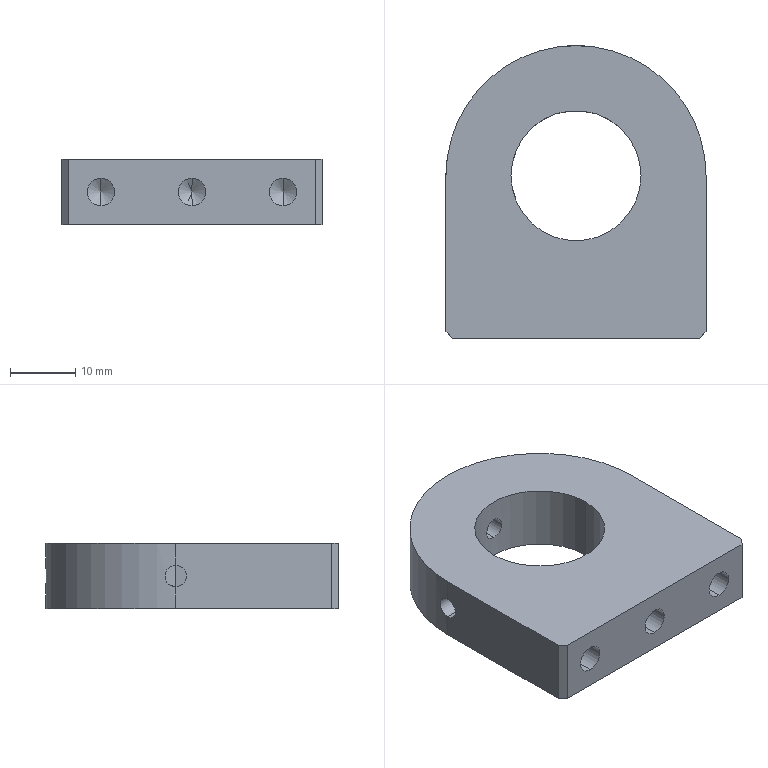Part | STEP file | MYT-A01-P11 | 1 solid | 27 faces | box 40 x 45 x 10 mm | volume 12427 mm3 | cylinder 14 | plane 7 | cone 6 | commonest cylinder face diameters 4.2 x6 3.3 x4 20 x2 40 x2
STEP:
#1=CARTESIAN_POINT('',(0.,35.,1.65));
#2=VERTEX_POINT('',#1);
#3=CARTESIAN_POINT('',(0.,35.,-1.65));
#4=VERTEX_POINT('',#3);
#5=CARTESIAN_POINT('',(0.,35.,1.65));
#6=CARTESIAN_POINT('',(-0.1092,35.,1.65));
#7=CARTESIAN_POINT('',(-0.2166,34.998,1.639));
#8=CARTESIAN_POINT('',(-0.4277,34.991,1.597));
#9=CARTESIAN_POINT('',(-0.5326,34.986,1.565));
#10=CARTESIAN_POINT('',(-0.7324,34.974,1.482));
#11=CARTESIAN_POINT('',(-0.8271,34.966,1.432));
#12=CARTESIAN_POINT('',(-1.006,34.95,1.312));
#13=CARTESIAN_POINT('',(-1.091,34.941,1.242));
#14=CARTESIAN_POINT('',(-1.319,34.914,1.014));
#15=CARTESIAN_POINT('',(-1.442,34.896,0.8307));
#16=CARTESIAN_POINT('',(-1.606,34.87,0.4337));
#17=CARTESIAN_POINT('',(-1.65,34.863,0.2163));
#18=CARTESIAN_POINT('',(-1.65,34.863,-0.1072));
#19=CARTESIAN_POINT('',(-1.639,34.865,-0.2167));
#20=CARTESIAN_POINT('',(-1.597,34.872,-0.4285));
#21=CARTESIAN_POINT('',(-1.566,34.877,-0.5315));
#22=CARTESIAN_POINT('',(-1.442,34.896,-0.8315));
#23=CARTESIAN_POINT('',(-1.32,34.914,-1.013));
#24=CARTESIAN_POINT('',(-1.09,34.941,-1.244));
#25=CARTESIAN_POINT('',(-1.007,34.95,-1.312));
#26=CARTESIAN_POINT('',(-0.8282,34.966,-1.431));
#27=CARTESIAN_POINT('',(-0.7316,34.974,-1.483));
#28=CARTESIAN_POINT('',(-0.532,34.986,-1.566));
#29=CARTESIAN_POINT('',(-0.4291,34.991,-1.597));
#30=CARTESIAN_POINT('',(-0.2173,34.998,-1.639));
#31=CARTESIAN_POINT('',(-0.1078,35.,-1.65));
#32=CARTESIAN_POINT('',(0.,35.,-1.65));
#33=B_SPLINE_CURVE_WITH_KNOTS('',3,(#5,#6,#7,#8,#9,#10,#11,#12,#13,#14,#15,#16,#17,#18,#19,#20,#21,#22,#23,#24,#25,#26,#27,#28,#29,#30,#31,#32),.UNSPECIFIED.,.F.,.F.,(4,2,2,2,2,2,2,2,2,2,2,2,2,4),(0.,0.000323,0.0006459,0.0009689,0.001292,0.001938,0.002584,0.002907,0.00323,0.003876,0.004199,0.004522,0.004845,0.005167),.UNSPECIFIED.);
#34=EDGE_CURVE('',#2,#4,#33,.T.);
#35=ORIENTED_EDGE('',*,*,#34,.T.);
#36=CARTESIAN_POINT('',(0.,45.,-1.65));
#37=VERTEX_POINT('',#36);
#38=CARTESIAN_POINT('',(0.,45.,-1.65));
#39=DIRECTION('',(0.,1.,0.));
#40=VECTOR('',#39,1000.);
#41=LINE('',#38,#40);
#42=EDGE_CURVE('',#4,#37,#41,.T.);
#43=ORIENTED_EDGE('',*,*,#42,.T.);
#44=CARTESIAN_POINT('',(0.,45.,1.65));
#45=VERTEX_POINT('',#44);
#46=CARTESIAN_POINT('',(0.,45.,-1.65));
#47=CARTESIAN_POINT('',(-0.109,45.,-1.65));
#48=CARTESIAN_POINT('',(-0.2163,44.999,-1.639));
#49=CARTESIAN_POINT('',(-0.4272,44.996,-1.597));
#50=CARTESIAN_POINT('',(-0.532,44.993,-1.566));
#51=CARTESIAN_POINT('',(-0.7318,44.987,-1.483));
#52=CARTESIAN_POINT('',(-0.8265,44.983,-1.432));
#53=CARTESIAN_POINT('',(-1.006,44.975,-1.312));
#54=CARTESIAN_POINT('',(-1.091,44.97,-1.243));
#55=CARTESIAN_POINT('',(-1.319,44.957,-1.015));
#56=CARTESIAN_POINT('',(-1.442,44.948,-0.8306));
#57=CARTESIAN_POINT('',(-1.606,44.936,-0.4336));
#58=CARTESIAN_POINT('',(-1.65,44.932,-0.2164));
#59=CARTESIAN_POINT('',(-1.65,44.932,0.1065));
#60=CARTESIAN_POINT('',(-1.639,44.933,0.2158));
#61=CARTESIAN_POINT('',(-1.597,44.936,0.4275));
#62=CARTESIAN_POINT('',(-1.566,44.939,0.5303));
#63=CARTESIAN_POINT('',(-1.484,44.945,0.7302));
#64=CARTESIAN_POINT('',(-1.432,44.949,0.8267));
#65=CARTESIAN_POINT('',(-1.313,44.957,1.006));
#66=CARTESIAN_POINT('',(-1.244,44.961,1.089));
#67=CARTESIAN_POINT('',(-1.091,44.97,1.243));
#68=CARTESIAN_POINT('',(-1.007,44.975,1.311));
#69=CARTESIAN_POINT('',(-0.8287,44.983,1.431));
#70=CARTESIAN_POINT('',(-0.7323,44.987,1.483));
#71=CARTESIAN_POINT('',(-0.4325,44.996,1.607));
#72=CARTESIAN_POINT('',(-0.2181,45.,1.65));
#73=CARTESIAN_POINT('',(0.,45.,1.65));
#74=B_SPLINE_CURVE_WITH_KNOTS('',3,(#46,#47,#48,#49,#50,#51,#52,#53,#54,#55,#56,#57,#58,#59,#60,#61,#62,#63,#64,#65,#66,#67,#68,#69,#70,#71,#72,#73),.UNSPECIFIED.,.F.,.F.,(4,2,2,2,2,2,2,2,2,2,2,2,2,4),(0.,0.0003225,0.000645,0.0009674,0.00129,0.001935,0.00258,0.002902,0.003225,0.003547,0.00387,0.004192,0.004515,0.00516),.UNSPECIFIED.);
#75=EDGE_CURVE('',#37,#45,#74,.T.);
#76=ORIENTED_EDGE('',*,*,#75,.T.);
#77=CARTESIAN_POINT('',(0.,45.,1.65));
#78=DIRECTION('',(0.,1.,0.));
#79=VECTOR('',#78,1000.);
#80=LINE('',#77,#79);
#81=EDGE_CURVE('',#2,#45,#80,.T.);
#82=ORIENTED_EDGE('',*,*,#81,.F.);
#83=EDGE_LOOP('',(#35,#43,#76,#82));
#84=FACE_OUTER_BOUND('',#83,.T.);
#85=CARTESIAN_POINT('',(0.,45.,0.));
#86=DIRECTION('',(0.,1.,0.));
#87=DIRECTION('',(0.,0.,1.));
#88=AXIS2_PLACEMENT_3D('',#85,#86,#87);
#89=CYLINDRICAL_SURFACE('',#88,1.65);
#90=ADVANCED_FACE('',(#84),#89,.F.);
#91=CARTESIAN_POINT('',(-10.,25.,1.65));
#92=VERTEX_POINT('',#91);
#93=CARTESIAN_POINT('',(-10.,25.,-1.65));
#94=VERTEX_POINT('',#93);
#95=CARTESIAN_POINT('',(-10.,25.,1.65));
#96=CARTESIAN_POINT('',(-10.,24.891,1.65));
#97=CARTESIAN_POINT('',(-9.998,24.783,1.639));
#98=CARTESIAN_POINT('',(-9.991,24.572,1.597));
#99=CARTESIAN_POINT('',(-9.986,24.467,1.565));
#100=CARTESIAN_POINT('',(-9.974,24.268,1.482));
#101=CARTESIAN_POINT('',(-9.966,24.173,1.432));
#102=CARTESIAN_POINT('',(-9.95,23.994,1.312));
#103=CARTESIAN_POINT('',(-9.941,23.909,1.242));
#104=CARTESIAN_POINT('',(-9.914,23.681,1.014));
#105=CARTESIAN_POINT('',(-9.896,23.558,0.8307));
#106=CARTESIAN_POINT('',(-9.87,23.394,0.4337));
#107=CARTESIAN_POINT('',(-9.863,23.35,0.2163));
#108=CARTESIAN_POINT('',(-9.863,23.35,-0.1072));
#109=CARTESIAN_POINT('',(-9.865,23.361,-0.2167));
#110=CARTESIAN_POINT('',(-9.872,23.403,-0.4285));
#111=CARTESIAN_POINT('',(-9.877,23.434,-0.5315));
#112=CARTESIAN_POINT('',(-9.896,23.558,-0.8315));
#113=CARTESIAN_POINT('',(-9.914,23.68,-1.013));
#114=CARTESIAN_POINT('',(-9.941,23.91,-1.244));
#115=CARTESIAN_POINT('',(-9.95,23.993,-1.312));
#116=CARTESIAN_POINT('',(-9.966,24.172,-1.431));
#117=CARTESIAN_POINT('',(-9.974,24.268,-1.483));
#118=CARTESIAN_POINT('',(-9.986,24.468,-1.566));
#119=CARTESIAN_POINT('',(-9.991,24.571,-1.597));
#120=CARTESIAN_POINT('',(-9.998,24.783,-1.639));
#121=CARTESIAN_POINT('',(-10.,24.892,-1.65));
#122=CARTESIAN_POINT('',(-10.,25.,-1.65));
#123=B_SPLINE_CURVE_WITH_KNOTS('',3,(#95,#96,#97,#98,#99,#100,#101,#102,#103,#104,#105,#106,#107,#108,#109,#110,#111,#112,#113,#114,#115,#116,#117,#118,#119,#120,#121,#122),.UNSPECIFIED.,.F.,.F.,(4,2,2,2,2,2,2,2,2,2,2,2,2,4),(0.,0.000323,0.0006459,0.0009689,0.001292,0.001938,0.002584,0.002907,0.00323,0.003876,0.004199,0.004522,0.004845,0.005167),.UNSPECIFIED.);
#124=EDGE_CURVE('',#92,#94,#123,.T.);
#125=ORIENTED_EDGE('',*,*,#124,.T.);
#126=CARTESIAN_POINT('',(-20.,25.,-1.65));
#127=VERTEX_POINT('',#126);
#128=CARTESIAN_POINT('',(-20.,25.,-1.65));
#129=DIRECTION('',(-1.,0.,0.));
#130=VECTOR('',#129,1000.);
#131=LINE('',#128,#130);
#132=EDGE_CURVE('',#94,#127,#131,.T.);
#133=ORIENTED_EDGE('',*,*,#132,.T.);
#134=CARTESIAN_POINT('',(-20.,25.,1.65));
#135=VERTEX_POINT('',#134);
#136=CARTESIAN_POINT('',(-20.,25.,0.));
#137=DIRECTION('',(-1.,0.,0.));
#138=DIRECTION('',(0.,0.,1.));
#139=AXIS2_PLACEMENT_3D('',#136,#137,#138);
#140=CIRCLE('',#139,1.65);
#141=EDGE_CURVE('',#127,#135,#140,.T.);
#142=ORIENTED_EDGE('',*,*,#141,.T.);
#143=CARTESIAN_POINT('',(-20.,25.,1.65));
#144=DIRECTION('',(-1.,0.,0.));
#145=VECTOR('',#144,1000.);
#146=LINE('',#143,#145);
#147=EDGE_CURVE('',#92,#135,#146,.T.);
#148=ORIENTED_EDGE('',*,*,#147,.F.);
#149=EDGE_LOOP('',(#125,#133,#142,#148));
#150=FACE_OUTER_BOUND('',#149,.T.);
#151=CARTESIAN_POINT('',(-20.,25.,0.));
#152=DIRECTION('',(-1.,0.,0.));
#153=DIRECTION('',(0.,0.,1.));
#154=AXIS2_PLACEMENT_3D('',#151,#152,#153);
#155=CYLINDRICAL_SURFACE('',#154,1.65);
#156=ADVANCED_FACE('',(#150),#155,.F.);
#157=CARTESIAN_POINT('',(-14.,12.4,2.1));
#158=VERTEX_POINT('',#157);
#159=CARTESIAN_POINT('',(-14.,12.4,-2.1));
#160=VERTEX_POINT('',#159);
#161=CARTESIAN_POINT('',(-14.,12.4,0.));
#162=DIRECTION('',(0.,-1.,0.));
#163=DIRECTION('',(0.,0.,-1.));
#164=AXIS2_PLACEMENT_3D('',#161,#162,#163);
#165=CIRCLE('',#164,2.1);
#166=EDGE_CURVE('',#158,#160,#165,.T.);
#167=ORIENTED_EDGE('',*,*,#166,.F.);
#168=CARTESIAN_POINT('',(-14.,0.,2.1));
#169=VERTEX_POINT('',#168);
#170=CARTESIAN_POINT('',(-14.,0.,2.1));
#171=DIRECTION('',(0.,-1.,0.));
#172=VECTOR('',#171,1000.);
#173=LINE('',#170,#172);
#174=EDGE_CURVE('',#158,#169,#173,.T.);
#175=ORIENTED_EDGE('',*,*,#174,.T.);
#176=CARTESIAN_POINT('',(-14.,0.,-2.1));
#177=VERTEX_POINT('',#176);
#178=CARTESIAN_POINT('',(-14.,0.,0.));
#179=DIRECTION('',(0.,-1.,0.));
#180=DIRECTION('',(0.,0.,-1.));
#181=AXIS2_PLACEMENT_3D('',#178,#179,#180);
#182=CIRCLE('',#181,2.1);
#183=EDGE_CURVE('',#169,#177,#182,.T.);
#184=ORIENTED_EDGE('',*,*,#183,.T.);
#185=CARTESIAN_POINT('',(-14.,0.,-2.1));
#186=DIRECTION('',(0.,-1.,0.));
#187=VECTOR('',#186,1000.);
#188=LINE('',#185,#187);
#189=EDGE_CURVE('',#160,#177,#188,.T.);
#190=ORIENTED_EDGE('',*,*,#189,.F.);
#191=EDGE_LOOP('',(#167,#175,#184,#190));
#192=FACE_OUTER_BOUND('',#191,.T.);
#193=CARTESIAN_POINT('',(-14.,0.,0.));
#194=DIRECTION('',(0.,-1.,0.));
#195=DIRECTION('',(0.,0.,-1.));
#196=AXIS2_PLACEMENT_3D('',#193,#194,#195);
#197=CYLINDRICAL_SURFACE('',#196,2.1);
#198=ADVANCED_FACE('',(#192),#197,.F.);
#199=CARTESIAN_POINT('',(-14.,13.662,0.));
#200=VERTEX_POINT('',#199);
#201=CARTESIAN_POINT('',(-14.,12.4,-2.1));
#202=DIRECTION('',(0.,-0.515,-0.8572));
#203=VECTOR('',#202,1000.);
#204=LINE('',#201,#203);
#205=EDGE_CURVE('',#200,#160,#204,.T.);
#206=ORIENTED_EDGE('',*,*,#205,.F.);
#207=CARTESIAN_POINT('',(-14.,12.4,2.1));
#208=DIRECTION('',(0.,-0.515,0.8572));
#209=VECTOR('',#208,1000.);
#210=LINE('',#207,#209);
#211=EDGE_CURVE('',#200,#158,#210,.T.);
#212=ORIENTED_EDGE('',*,*,#211,.T.);
#213=ORIENTED_EDGE('',*,*,#166,.T.);
#214=EDGE_LOOP('',(#206,#212,#213));
#215=FACE_OUTER_BOUND('',#214,.T.);
#216=CARTESIAN_POINT('',(-14.,12.4,0.));
#217=DIRECTION('',(0.,-1.,0.));
#218=DIRECTION('',(0.,0.,-1.));
#219=AXIS2_PLACEMENT_3D('',#216,#217,#218);
#220=CONICAL_SURFACE('',#219,2.1,1.03);
#221=ADVANCED_FACE('',(#215),#220,.F.);
#222=CARTESIAN_POINT('',(0.,12.4,2.1));
#223=VERTEX_POINT('',#222);
#224=CARTESIAN_POINT('',(0.,12.4,-2.1));
#225=VERTEX_POINT('',#224);
#226=CARTESIAN_POINT('',(0.,12.4,0.));
#227=DIRECTION('',(0.,-1.,0.));
#228=DIRECTION('',(0.,0.,-1.));
#229=AXIS2_PLACEMENT_3D('',#226,#227,#228);
#230=CIRCLE('',#229,2.1);
#231=EDGE_CURVE('',#223,#225,#230,.T.);
#232=ORIENTED_EDGE('',*,*,#231,.F.);
#233=CARTESIAN_POINT('',(0.,0.,2.1));
#234=VERTEX_POINT('',#233);
#235=CARTESIAN_POINT('',(0.,0.,2.1));
#236=DIRECTION('',(0.,-1.,0.));
#237=VECTOR('',#236,1000.);
#238=LINE('',#235,#237);
#239=EDGE_CURVE('',#223,#234,#238,.T.);
#240=ORIENTED_EDGE('',*,*,#239,.T.);
#241=CARTESIAN_POINT('',(0.,0.,-2.1));
#242=VERTEX_POINT('',#241);
#243=CARTESIAN_POINT('',(0.,0.,0.));
#244=DIRECTION('',(0.,-1.,0.));
#245=DIRECTION('',(0.,0.,-1.));
#246=AXIS2_PLACEMENT_3D('',#243,#244,#245);
#247=CIRCLE('',#246,2.1);
#248=EDGE_CURVE('',#234,#242,#247,.T.);
#249=ORIENTED_EDGE('',*,*,#248,.T.);
#250=CARTESIAN_POINT('',(0.,0.,-2.1));
#251=DIRECTION('',(0.,-1.,0.));
#252=VECTOR('',#251,1000.);
#253=LINE('',#250,#252);
#254=EDGE_CURVE('',#225,#242,#253,.T.);
#255=ORIENTED_EDGE('',*,*,#254,.F.);
#256=EDGE_LOOP('',(#232,#240,#249,#255));
#257=FACE_OUTER_BOUND('',#256,.T.);
#258=CARTESIAN_POINT('',(0.,0.,0.));
#259=DIRECTION('',(0.,-1.,0.));
#260=DIRECTION('',(0.,0.,-1.));
#261=AXIS2_PLACEMENT_3D('',#258,#259,#260);
#262=CYLINDRICAL_SURFACE('',#261,2.1);
#263=ADVANCED_FACE('',(#257),#262,.F.);
#264=CARTESIAN_POINT('',(0.,13.662,0.));
#265=VERTEX_POINT('',#264);
#266=CARTESIAN_POINT('',(0.,12.4,-2.1));
#267=DIRECTION('',(0.,-0.515,-0.8572));
#268=VECTOR('',#267,1000.);
#269=LINE('',#266,#268);
#270=EDGE_CURVE('',#265,#225,#269,.T.);
#271=ORIENTED_EDGE('',*,*,#270,.F.);
#272=CARTESIAN_POINT('',(0.,12.4,2.1));
#273=DIRECTION('',(0.,-0.515,0.8572));
#274=VECTOR('',#273,1000.);
#275=LINE('',#272,#274);
#276=EDGE_CURVE('',#265,#223,#275,.T.);
#277=ORIENTED_EDGE('',*,*,#276,.T.);
#278=ORIENTED_EDGE('',*,*,#231,.T.);
#279=EDGE_LOOP('',(#271,#277,#278));
#280=FACE_OUTER_BOUND('',#279,.T.);
#281=CARTESIAN_POINT('',(0.,12.4,0.));
#282=DIRECTION('',(0.,-1.,0.));
#283=DIRECTION('',(0.,0.,-1.));
#284=AXIS2_PLACEMENT_3D('',#281,#282,#283);
#285=CONICAL_SURFACE('',#284,2.1,1.03);
#286=ADVANCED_FACE('',(#280),#285,.F.);
#287=CARTESIAN_POINT('',(14.,12.4,2.1));
#288=VERTEX_POINT('',#287);
#289=CARTESIAN_POINT('',(14.,12.4,-2.1));
#290=VERTEX_POINT('',#289);
#291=CARTESIAN_POINT('',(14.,12.4,0.));
#292=DIRECTION('',(0.,-1.,0.));
#293=DIRECTION('',(0.,0.,-1.));
#294=AXIS2_PLACEMENT_3D('',#291,#292,#293);
#295=CIRCLE('',#294,2.1);
#296=EDGE_CURVE('',#288,#290,#295,.T.);
#297=ORIENTED_EDGE('',*,*,#296,.F.);
#298=CARTESIAN_POINT('',(14.,0.,2.1));
#299=VERTEX_POINT('',#298);
#300=CARTESIAN_POINT('',(14.,0.,2.1));
#301=DIRECTION('',(0.,-1.,0.));
#302=VECTOR('',#301,1000.);
#303=LINE('',#300,#302);
#304=EDGE_CURVE('',#288,#299,#303,.T.);
#305=ORIENTED_EDGE('',*,*,#304,.T.);
#306=CARTESIAN_POINT('',(14.,0.,-2.1));
#307=VERTEX_POINT('',#306);
#308=CARTESIAN_POINT('',(14.,0.,0.));
#309=DIRECTION('',(0.,-1.,0.));
#310=DIRECTION('',(0.,0.,-1.));
#311=AXIS2_PLACEMENT_3D('',#308,#309,#310);
#312=CIRCLE('',#311,2.1);
#313=EDGE_CURVE('',#299,#307,#312,.T.);
#314=ORIENTED_EDGE('',*,*,#313,.T.);
#315=CARTESIAN_POINT('',(14.,0.,-2.1));
#316=DIRECTION('',(0.,-1.,0.));
#317=VECTOR('',#316,1000.);
#318=LINE('',#315,#317);
#319=EDGE_CURVE('',#290,#307,#318,.T.);
#320=ORIENTED_EDGE('',*,*,#319,.F.);
#321=EDGE_LOOP('',(#297,#305,#314,#320));
#322=FACE_OUTER_BOUND('',#321,.T.);
#323=CARTESIAN_POINT('',(14.,0.,0.));
#324=DIRECTION('',(0.,-1.,0.));
#325=DIRECTION('',(0.,0.,-1.));
#326=AXIS2_PLACEMENT_3D('',#323,#324,#325);
#327=CYLINDRICAL_SURFACE('',#326,2.1);
#328=ADVANCED_FACE('',(#322),#327,.F.);
#329=CARTESIAN_POINT('',(14.,13.662,0.));
#330=VERTEX_POINT('',#329);
#331=CARTESIAN_POINT('',(14.,12.4,-2.1));
#332=DIRECTION('',(0.,-0.515,-0.8572));
#333=VECTOR('',#332,1000.);
#334=LINE('',#331,#333);
#335=EDGE_CURVE('',#330,#290,#334,.T.);
#336=ORIENTED_EDGE('',*,*,#335,.F.);
#337=CARTESIAN_POINT('',(14.,12.4,2.1));
#338=DIRECTION('',(0.,-0.515,0.8572));
#339=VECTOR('',#338,1000.);
#340=LINE('',#337,#339);
#341=EDGE_CURVE('',#330,#288,#340,.T.);
#342=ORIENTED_EDGE('',*,*,#341,.T.);
#343=ORIENTED_EDGE('',*,*,#296,.T.);
#344=EDGE_LOOP('',(#336,#342,#343));
#345=FACE_OUTER_BOUND('',#344,.T.);
#346=CARTESIAN_POINT('',(14.,12.4,0.));
#347=DIRECTION('',(0.,-1.,0.));
#348=DIRECTION('',(0.,0.,-1.));
#349=AXIS2_PLACEMENT_3D('',#346,#347,#348);
#350=CONICAL_SURFACE('',#349,2.1,1.03);
#351=ADVANCED_FACE('',(#345),#350,.F.);
#352=CARTESIAN_POINT('',(-10.,25.,5.));
#353=VERTEX_POINT('',#352);
#354=CARTESIAN_POINT('',(10.,25.,5.));
#355=VERTEX_POINT('',#354);
#356=CARTESIAN_POINT('',(0.,25.,5.));
#357=DIRECTION('',(0.,0.,1.));
#358=DIRECTION('',(1.,0.,0.));
#359=AXIS2_PLACEMENT_3D('',#356,#357,#358);
#360=CIRCLE('',#359,10.);
#361=EDGE_CURVE('',#353,#355,#360,.T.);
#362=ORIENTED_EDGE('',*,*,#361,.T.);
#363=CARTESIAN_POINT('',(10.,25.,-5.));
#364=VERTEX_POINT('',#363);
#365=CARTESIAN_POINT('',(10.,25.,5.));
#366=DIRECTION('',(0.,0.,-1.));
#367=VECTOR('',#366,1000.);
#368=LINE('',#365,#367);
#369=EDGE_CURVE('',#355,#364,#368,.T.);
#370=ORIENTED_EDGE('',*,*,#369,.T.);
#371=CARTESIAN_POINT('',(-10.,25.,-5.));
#372=VERTEX_POINT('',#371);
#373=CARTESIAN_POINT('',(0.,25.,-5.));
#374=DIRECTION('',(0.,0.,1.));
#375=DIRECTION('',(1.,0.,0.));
#376=AXIS2_PLACEMENT_3D('',#373,#374,#375);
#377=CIRCLE('',#376,10.);
#378=EDGE_CURVE('',#372,#364,#377,.T.);
#379=ORIENTED_EDGE('',*,*,#378,.F.);
#380=CARTESIAN_POINT('',(-10.,25.,5.));
#381=DIRECTION('',(0.,0.,-1.));
#382=VECTOR('',#381,1000.);
#383=LINE('',#380,#382);
#384=EDGE_CURVE('',#94,#372,#383,.T.);
#385=ORIENTED_EDGE('',*,*,#384,.F.);
#386=ORIENTED_EDGE('',*,*,#124,.F.);
#387=CARTESIAN_POINT('',(-10.,25.,5.));
#388=DIRECTION('',(0.,0.,-1.));
#389=VECTOR('',#388,1000.);
#390=LINE('',#387,#389);
#391=EDGE_CURVE('',#353,#92,#390,.T.);
#392=ORIENTED_EDGE('',*,*,#391,.F.);
#393=EDGE_LOOP('',(#362,#370,#379,#385,#386,#392));
#394=FACE_OUTER_BOUND('',#393,.T.);
#395=CARTESIAN_POINT('',(0.,25.,5.));
#396=DIRECTION('',(0.,0.,-1.));
#397=DIRECTION('',(-1.,0.,0.));
#398=AXIS2_PLACEMENT_3D('',#395,#396,#397);
#399=CYLINDRICAL_SURFACE('',#398,10.);
#400=ADVANCED_FACE('',(#394),#399,.F.);
#401=CARTESIAN_POINT('',(-19.,0.,5.));
#402=VERTEX_POINT('',#401);
#403=CARTESIAN_POINT('',(19.,0.,5.));
#404=VERTEX_POINT('',#403);
#405=CARTESIAN_POINT('',(-20.,0.,5.));
#406=DIRECTION('',(1.,0.,0.));
#407=VECTOR('',#406,1000.);
#408=LINE('',#405,#407);
#409=EDGE_CURVE('',#402,#404,#408,.T.);
#410=ORIENTED_EDGE('',*,*,#409,.T.);
#411=CARTESIAN_POINT('',(20.,1.,5.));
#412=VERTEX_POINT('',#411);
#413=CARTESIAN_POINT('',(9.5,-9.5,5.));
#414=DIRECTION('',(0.7071,0.7071,0.));
#415=VECTOR('',#414,1000.);
#416=LINE('',#413,#415);
#417=EDGE_CURVE('',#404,#412,#416,.T.);
#418=ORIENTED_EDGE('',*,*,#417,.T.);
#419=CARTESIAN_POINT('',(20.,25.,5.));
#420=VERTEX_POINT('',#419);
#421=CARTESIAN_POINT('',(20.,45.,5.));
#422=DIRECTION('',(0.,1.,0.));
#423=VECTOR('',#422,1000.);
#424=LINE('',#421,#423);
#425=EDGE_CURVE('',#412,#420,#424,.T.);
#426=ORIENTED_EDGE('',*,*,#425,.T.);
#427=CARTESIAN_POINT('',(0.,45.,5.));
#428=VERTEX_POINT('',#427);
#429=CARTESIAN_POINT('',(0.,25.,5.));
#430=DIRECTION('',(0.,0.,1.));
#431=DIRECTION('',(1.,0.,0.));
#432=AXIS2_PLACEMENT_3D('',#429,#430,#431);
#433=CIRCLE('',#432,20.);
#434=EDGE_CURVE('',#420,#428,#433,.T.);
#435=ORIENTED_EDGE('',*,*,#434,.T.);
#436=CARTESIAN_POINT('',(-20.,25.,5.));
#437=VERTEX_POINT('',#436);
#438=CARTESIAN_POINT('',(0.,25.,5.));
#439=DIRECTION('',(0.,0.,1.));
#440=DIRECTION('',(1.,0.,0.));
#441=AXIS2_PLACEMENT_3D('',#438,#439,#440);
#442=CIRCLE('',#441,20.);
#443=EDGE_CURVE('',#428,#437,#442,.T.);
#444=ORIENTED_EDGE('',*,*,#443,.T.);
#445=CARTESIAN_POINT('',(-20.,1.,5.));
#446=VERTEX_POINT('',#445);
#447=CARTESIAN_POINT('',(-20.,45.,5.));
#448=DIRECTION('',(0.,-1.,0.));
#449=VECTOR('',#448,1000.);
#450=LINE('',#447,#449);
#451=EDGE_CURVE('',#437,#446,#450,.T.);
#452=ORIENTED_EDGE('',*,*,#451,.T.);
#453=CARTESIAN_POINT('',(-9.5,-9.5,5.));
#454=DIRECTION('',(0.7071,-0.7071,0.));
#455=VECTOR('',#454,1000.);
#456=LINE('',#453,#455);
#457=EDGE_CURVE('',#446,#402,#456,.T.);
#458=ORIENTED_EDGE('',*,*,#457,.T.);
#459=EDGE_LOOP('',(#410,#418,#426,#435,#444,#452,#458));
#460=FACE_OUTER_BOUND('',#459,.T.);
#461=ORIENTED_EDGE('',*,*,#361,.F.);
#462=CARTESIAN_POINT('',(0.,25.,5.));
#463=DIRECTION('',(0.,0.,1.));
#464=DIRECTION('',(1.,0.,0.));
#465=AXIS2_PLACEMENT_3D('',#462,#463,#464);
#466=CIRCLE('',#465,10.);
#467=EDGE_CURVE('',#355,#353,#466,.T.);
#468=ORIENTED_EDGE('',*,*,#467,.F.);
#469=EDGE_LOOP('',(#461,#468));
#470=FACE_BOUND('',#469,.T.);
#471=CARTESIAN_POINT('',(0.,0.,5.));
#472=DIRECTION('',(0.,0.,1.));
#473=DIRECTION('',(1.,0.,0.));
#474=AXIS2_PLACEMENT_3D('',#471,#472,#473);
#475=PLANE('',#474);
#476=ADVANCED_FACE('',(#460,#470),#475,.T.);
#477=CARTESIAN_POINT('',(20.,1.,-5.));
#478=VERTEX_POINT('',#477);
#479=CARTESIAN_POINT('',(20.,25.,-5.));
#480=VERTEX_POINT('',#479);
#481=CARTESIAN_POINT('',(20.,45.,-5.));
#482=DIRECTION('',(0.,1.,0.));
#483=VECTOR('',#482,1000.);
#484=LINE('',#481,#483);
#485=EDGE_CURVE('',#478,#480,#484,.T.);
#486=ORIENTED_EDGE('',*,*,#485,.F.);
#487=CARTESIAN_POINT('',(19.,0.,-5.));
#488=VERTEX_POINT('',#487);
#489=CARTESIAN_POINT('',(20.,1.,-5.));
#490=DIRECTION('',(-0.7071,-0.7071,0.));
#491=VECTOR('',#490,1000.);
#492=LINE('',#489,#491);
#493=EDGE_CURVE('',#478,#488,#492,.T.);
#494=ORIENTED_EDGE('',*,*,#493,.T.);
#495=CARTESIAN_POINT('',(-19.,0.,-5.));
#496=VERTEX_POINT('',#495);
#497=CARTESIAN_POINT('',(-20.,0.,-5.));
#498=DIRECTION('',(1.,0.,0.));
#499=VECTOR('',#498,1000.);
#500=LINE('',#497,#499);
#501=EDGE_CURVE('',#496,#488,#500,.T.);
#502=ORIENTED_EDGE('',*,*,#501,.F.);
#503=CARTESIAN_POINT('',(-20.,1.,-5.));
#504=VERTEX_POINT('',#503);
#505=CARTESIAN_POINT('',(-19.,0.,-5.));
#506=DIRECTION('',(-0.7071,0.7071,0.));
#507=VECTOR('',#506,1000.);
#508=LINE('',#505,#507);
#509=EDGE_CURVE('',#496,#504,#508,.T.);
#510=ORIENTED_EDGE('',*,*,#509,.T.);
#511=CARTESIAN_POINT('',(-20.,25.,-5.));
#512=VERTEX_POINT('',#511);
#513=CARTESIAN_POINT('',(-20.,45.,-5.));
#514=DIRECTION('',(0.,-1.,0.));
#515=VECTOR('',#514,1000.);
#516=LINE('',#513,#515);
#517=EDGE_CURVE('',#512,#504,#516,.T.);
#518=ORIENTED_EDGE('',*,*,#517,.F.);
#519=CARTESIAN_POINT('',(0.,45.,-5.));
#520=VERTEX_POINT('',#519);
#521=CARTESIAN_POINT('',(0.,25.,-5.));
#522=DIRECTION('',(0.,0.,-1.));
#523=DIRECTION('',(1.,0.,0.));
#524=AXIS2_PLACEMENT_3D('',#521,#522,#523);
#525=CIRCLE('',#524,20.);
#526=EDGE_CURVE('',#512,#520,#525,.T.);
#527=ORIENTED_EDGE('',*,*,#526,.T.);
#528=CARTESIAN_POINT('',(0.,25.,-5.));
#529=DIRECTION('',(0.,0.,-1.));
#530=DIRECTION('',(1.,0.,0.));
#531=AXIS2_PLACEMENT_3D('',#528,#529,#530);
#532=CIRCLE('',#531,20.);
#533=EDGE_CURVE('',#520,#480,#532,.T.);
#534=ORIENTED_EDGE('',*,*,#533,.T.);
#535=EDGE_LOOP('',(#486,#494,#502,#510,#518,#527,#534));
#536=FACE_OUTER_BOUND('',#535,.T.);
#537=ORIENTED_EDGE('',*,*,#378,.T.);
#538=CARTESIAN_POINT('',(0.,25.,-5.));
#539=DIRECTION('',(0.,0.,1.));
#540=DIRECTION('',(1.,0.,0.));
#541=AXIS2_PLACEMENT_3D('',#538,#539,#540);
#542=CIRCLE('',#541,10.);
#543=EDGE_CURVE('',#364,#372,#542,.T.);
#544=ORIENTED_EDGE('',*,*,#543,.T.);
#545=EDGE_LOOP('',(#537,#544));
#546=FACE_BOUND('',#545,.T.);
#547=CARTESIAN_POINT('',(0.,0.,-5.));
#548=DIRECTION('',(0.,0.,1.));
#549=DIRECTION('',(1.,0.,0.));
#550=AXIS2_PLACEMENT_3D('',#547,#548,#549);
#551=PLANE('',#550);
#552=ADVANCED_FACE('',(#536,#546),#551,.F.);
#553=CARTESIAN_POINT('',(-20.,25.,5.));
#554=DIRECTION('',(0.,0.,-1.));
#555=VECTOR('',#554,1000.);
#556=LINE('',#553,#555);
#557=EDGE_CURVE('',#437,#135,#556,.T.);
#558=ORIENTED_EDGE('',*,*,#557,.T.);
#559=ORIENTED_EDGE('',*,*,#141,.F.);
#560=CARTESIAN_POINT('',(-20.,25.,5.));
#561=DIRECTION('',(0.,0.,-1.));
#562=VECTOR('',#561,1000.);
#563=LINE('',#560,#562);
#564=EDGE_CURVE('',#127,#512,#563,.T.);
#565=ORIENTED_EDGE('',*,*,#564,.T.);
#566=ORIENTED_EDGE('',*,*,#517,.T.);
#567=CARTESIAN_POINT('',(-20.,1.,5.));
#568=DIRECTION('',(0.,0.,1.));
#569=VECTOR('',#568,1000.);
#570=LINE('',#567,#569);
#571=EDGE_CURVE('',#504,#446,#570,.T.);
#572=ORIENTED_EDGE('',*,*,#571,.T.);
#573=ORIENTED_EDGE('',*,*,#451,.F.);
#574=EDGE_LOOP('',(#558,#559,#565,#566,#572,#573));
#575=FACE_OUTER_BOUND('',#574,.T.);
#576=CARTESIAN_POINT('',(-20.,45.,5.));
#577=DIRECTION('',(1.,0.,0.));
#578=DIRECTION('',(0.,1.,0.));
#579=AXIS2_PLACEMENT_3D('',#576,#577,#578);
#580=PLANE('',#579);
#581=ADVANCED_FACE('',(#575),#580,.F.);
#582=CARTESIAN_POINT('',(-14.,0.,0.));
#583=DIRECTION('',(0.,-1.,0.));
#584=DIRECTION('',(0.,0.,-1.));
#585=AXIS2_PLACEMENT_3D('',#582,#583,#584);
#586=CIRCLE('',#585,2.1);
#587=EDGE_CURVE('',#177,#169,#586,.T.);
#588=ORIENTED_EDGE('',*,*,#587,.F.);
#589=ORIENTED_EDGE('',*,*,#183,.F.);
#590=EDGE_LOOP('',(#588,#589));
#591=FACE_BOUND('',#590,.T.);
#592=CARTESIAN_POINT('',(0.,0.,0.));
#593=DIRECTION('',(0.,-1.,0.));
#594=DIRECTION('',(0.,0.,-1.));
#595=AXIS2_PLACEMENT_3D('',#592,#593,#594);
#596=CIRCLE('',#595,2.1);
#597=EDGE_CURVE('',#242,#234,#596,.T.);
#598=ORIENTED_EDGE('',*,*,#597,.F.);
#599=ORIENTED_EDGE('',*,*,#248,.F.);
#600=EDGE_LOOP('',(#598,#599));
#601=FACE_BOUND('',#600,.T.);
#602=CARTESIAN_POINT('',(14.,0.,0.));
#603=DIRECTION('',(0.,-1.,0.));
#604=DIRECTION('',(0.,0.,-1.));
#605=AXIS2_PLACEMENT_3D('',#602,#603,#604);
#606=CIRCLE('',#605,2.1);
#607=EDGE_CURVE('',#307,#299,#606,.T.);
#608=ORIENTED_EDGE('',*,*,#607,.F.);
#609=ORIENTED_EDGE('',*,*,#313,.F.);
#610=EDGE_LOOP('',(#608,#609));
#611=FACE_BOUND('',#610,.T.);
#612=ORIENTED_EDGE('',*,*,#501,.T.);
#613=CARTESIAN_POINT('',(19.,0.,5.));
#614=DIRECTION('',(0.,0.,1.));
#615=VECTOR('',#614,1000.);
#616=LINE('',#613,#615);
#617=EDGE_CURVE('',#488,#404,#616,.T.);
#618=ORIENTED_EDGE('',*,*,#617,.T.);
#619=ORIENTED_EDGE('',*,*,#409,.F.);
#620=CARTESIAN_POINT('',(-19.,0.,5.));
#621=DIRECTION('',(0.,0.,-1.));
#622=VECTOR('',#621,1000.);
#623=LINE('',#620,#622);
#624=EDGE_CURVE('',#402,#496,#623,.T.);
#625=ORIENTED_EDGE('',*,*,#624,.T.);
#626=EDGE_LOOP('',(#612,#618,#619,#625));
#627=FACE_OUTER_BOUND('',#626,.T.);
#628=CARTESIAN_POINT('',(-20.,0.,5.));
#629=DIRECTION('',(0.,1.,0.));
#630=DIRECTION('',(0.,0.,1.));
#631=AXIS2_PLACEMENT_3D('',#628,#629,#630);
#632=PLANE('',#631);
#633=ADVANCED_FACE('',(#591,#601,#611,#627),#632,.F.);
#634=ORIENTED_EDGE('',*,*,#425,.F.);
#635=CARTESIAN_POINT('',(20.,1.,5.));
#636=DIRECTION('',(0.,0.,-1.));
#637=VECTOR('',#636,1000.);
#638=LINE('',#635,#637);
#639=EDGE_CURVE('',#412,#478,#638,.T.);
#640=ORIENTED_EDGE('',*,*,#639,.T.);
#641=ORIENTED_EDGE('',*,*,#485,.T.);
#642=CARTESIAN_POINT('',(20.,25.,5.));
#643=DIRECTION('',(0.,0.,1.));
#644=VECTOR('',#643,1000.);
#645=LINE('',#642,#644);
#646=EDGE_CURVE('',#480,#420,#645,.T.);
#647=ORIENTED_EDGE('',*,*,#646,.T.);
#648=EDGE_LOOP('',(#634,#640,#641,#647));
#649=FACE_OUTER_BOUND('',#648,.T.);
#650=CARTESIAN_POINT('',(20.,45.,5.));
#651=DIRECTION('',(-1.,0.,0.));
#652=DIRECTION('',(0.,-1.,0.));
#653=AXIS2_PLACEMENT_3D('',#650,#651,#652);
#654=PLANE('',#653);
#655=ADVANCED_FACE('',(#649),#654,.F.);
#656=ORIENTED_EDGE('',*,*,#369,.F.);
#657=ORIENTED_EDGE('',*,*,#467,.T.);
#658=ORIENTED_EDGE('',*,*,#391,.T.);
#659=CARTESIAN_POINT('',(-10.,25.,-1.65));
#660=CARTESIAN_POINT('',(-10.,25.216,-1.65));
#661=CARTESIAN_POINT('',(-9.993,25.433,-1.607));
#662=CARTESIAN_POINT('',(-9.967,25.83,-1.442));
#663=CARTESIAN_POINT('',(-9.95,26.014,-1.319));
#664=CARTESIAN_POINT('',(-9.923,26.242,-1.091));
#665=CARTESIAN_POINT('',(-9.914,26.312,-1.007));
#666=CARTESIAN_POINT('',(-9.897,26.431,-0.8279));
#667=CARTESIAN_POINT('',(-9.89,26.482,-0.7333));
#668=CARTESIAN_POINT('',(-9.87,26.607,-0.4334));
#669=CARTESIAN_POINT('',(-9.863,26.65,-0.219));
#670=CARTESIAN_POINT('',(-9.863,26.65,0.108));
#671=CARTESIAN_POINT('',(-9.865,26.639,0.2153));
#672=CARTESIAN_POINT('',(-9.872,26.598,0.4265));
#673=CARTESIAN_POINT('',(-9.877,26.566,0.5316));
#674=CARTESIAN_POINT('',(-9.889,26.483,0.7311));
#675=CARTESIAN_POINT('',(-9.897,26.433,0.8259));
#676=CARTESIAN_POINT('',(-9.914,26.313,1.005));
#677=CARTESIAN_POINT('',(-9.923,26.243,1.09));
#678=CARTESIAN_POINT('',(-9.949,26.016,1.318));
#679=CARTESIAN_POINT('',(-9.967,25.832,1.441));
#680=CARTESIAN_POINT('',(-9.992,25.435,1.606));
#681=CARTESIAN_POINT('',(-10.,25.218,1.65));
#682=CARTESIAN_POINT('',(-10.,25.,1.65));
#683=B_SPLINE_CURVE_WITH_KNOTS('',3,(#659,#660,#661,#662,#663,#664,#665,#666,#667,#668,#669,#670,#671,#672,#673,#674,#675,#676,#677,#678,#679,#680,#681,#682),.UNSPECIFIED.,.F.,.F.,(4,2,2,2,2,2,2,2,2,2,2,4),(0.005167,0.005813,0.006459,0.006782,0.007105,0.007751,0.008073,0.008396,0.008719,0.009042,0.009688,0.01033),.UNSPECIFIED.);
#684=EDGE_CURVE('',#94,#92,#683,.T.);
#685=ORIENTED_EDGE('',*,*,#684,.F.);
#686=ORIENTED_EDGE('',*,*,#384,.T.);
#687=ORIENTED_EDGE('',*,*,#543,.F.);
#688=EDGE_LOOP('',(#656,#657,#658,#685,#686,#687));
#689=FACE_OUTER_BOUND('',#688,.T.);
#690=ORIENTED_EDGE('',*,*,#34,.F.);
#691=CARTESIAN_POINT('',(0.,35.,-1.65));
#692=CARTESIAN_POINT('',(0.2155,35.,-1.65));
#693=CARTESIAN_POINT('',(0.4329,34.993,-1.607));
#694=CARTESIAN_POINT('',(0.8301,34.967,-1.442));
#695=CARTESIAN_POINT('',(1.014,34.95,-1.319));
#696=CARTESIAN_POINT('',(1.242,34.923,-1.091));
#697=CARTESIAN_POINT('',(1.312,34.914,-1.007));
#698=CARTESIAN_POINT('',(1.431,34.897,-0.8279));
#699=CARTESIAN_POINT('',(1.482,34.89,-0.7333));
#700=CARTESIAN_POINT('',(1.607,34.87,-0.4334));
#701=CARTESIAN_POINT('',(1.65,34.863,-0.219));
#702=CARTESIAN_POINT('',(1.65,34.863,0.108));
#703=CARTESIAN_POINT('',(1.639,34.865,0.2153));
#704=CARTESIAN_POINT('',(1.598,34.872,0.4265));
#705=CARTESIAN_POINT('',(1.566,34.877,0.5316));
#706=CARTESIAN_POINT('',(1.483,34.889,0.7311));
#707=CARTESIAN_POINT('',(1.433,34.897,0.8259));
#708=CARTESIAN_POINT('',(1.313,34.914,1.005));
#709=CARTESIAN_POINT('',(1.243,34.923,1.09));
#710=CARTESIAN_POINT('',(1.016,34.949,1.318));
#711=CARTESIAN_POINT('',(0.8321,34.967,1.441));
#712=CARTESIAN_POINT('',(0.4353,34.992,1.606));
#713=CARTESIAN_POINT('',(0.2184,35.,1.65));
#714=CARTESIAN_POINT('',(0.,35.,1.65));
#715=B_SPLINE_CURVE_WITH_KNOTS('',3,(#691,#692,#693,#694,#695,#696,#697,#698,#699,#700,#701,#702,#703,#704,#705,#706,#707,#708,#709,#710,#711,#712,#713,#714),.UNSPECIFIED.,.F.,.F.,(4,2,2,2,2,2,2,2,2,2,2,4),(0.005167,0.005813,0.006459,0.006782,0.007105,0.007751,0.008073,0.008396,0.008719,0.009042,0.009688,0.01033),.UNSPECIFIED.);
#716=EDGE_CURVE('',#4,#2,#715,.T.);
#717=ORIENTED_EDGE('',*,*,#716,.F.);
#718=EDGE_LOOP('',(#690,#717));
#719=FACE_BOUND('',#718,.T.);
#720=CARTESIAN_POINT('',(0.,25.,5.));
#721=DIRECTION('',(0.,0.,-1.));
#722=DIRECTION('',(-1.,0.,0.));
#723=AXIS2_PLACEMENT_3D('',#720,#721,#722);
#724=CYLINDRICAL_SURFACE('',#723,10.);
#725=ADVANCED_FACE('',(#689,#719),#724,.F.);
#726=ORIENTED_EDGE('',*,*,#75,.F.);
#727=CARTESIAN_POINT('',(0.,45.,5.));
#728=DIRECTION('',(0.,0.,1.));
#729=VECTOR('',#728,1000.);
#730=LINE('',#727,#729);
#731=EDGE_CURVE('',#520,#37,#730,.T.);
#732=ORIENTED_EDGE('',*,*,#731,.F.);
#733=ORIENTED_EDGE('',*,*,#526,.F.);
#734=ORIENTED_EDGE('',*,*,#564,.F.);
#735=CARTESIAN_POINT('',(-20.,25.,1.65));
#736=CARTESIAN_POINT('',(-20.,25.109,1.65));
#737=CARTESIAN_POINT('',(-19.999,25.216,1.639));
#738=CARTESIAN_POINT('',(-19.996,25.427,1.597));
#739=CARTESIAN_POINT('',(-19.993,25.532,1.566));
#740=CARTESIAN_POINT('',(-19.987,25.732,1.483));
#741=CARTESIAN_POINT('',(-19.983,25.827,1.432));
#742=CARTESIAN_POINT('',(-19.975,26.006,1.312));
#743=CARTESIAN_POINT('',(-19.97,26.091,1.243));
#744=CARTESIAN_POINT('',(-19.957,26.319,1.015));
#745=CARTESIAN_POINT('',(-19.948,26.442,0.8306));
#746=CARTESIAN_POINT('',(-19.936,26.606,0.4336));
#747=CARTESIAN_POINT('',(-19.932,26.65,0.2164));
#748=CARTESIAN_POINT('',(-19.932,26.65,-0.1065));
#749=CARTESIAN_POINT('',(-19.933,26.639,-0.2158));
#750=CARTESIAN_POINT('',(-19.936,26.597,-0.4275));
#751=CARTESIAN_POINT('',(-19.939,26.566,-0.5303));
#752=CARTESIAN_POINT('',(-19.945,26.484,-0.7302));
#753=CARTESIAN_POINT('',(-19.949,26.432,-0.8267));
#754=CARTESIAN_POINT('',(-19.957,26.313,-1.006));
#755=CARTESIAN_POINT('',(-19.961,26.244,-1.089));
#756=CARTESIAN_POINT('',(-19.97,26.091,-1.243));
#757=CARTESIAN_POINT('',(-19.975,26.007,-1.311));
#758=CARTESIAN_POINT('',(-19.983,25.829,-1.431));
#759=CARTESIAN_POINT('',(-19.987,25.732,-1.483));
#760=CARTESIAN_POINT('',(-19.996,25.433,-1.607));
#761=CARTESIAN_POINT('',(-20.,25.218,-1.65));
#762=CARTESIAN_POINT('',(-20.,25.,-1.65));
#763=B_SPLINE_CURVE_WITH_KNOTS('',3,(#735,#736,#737,#738,#739,#740,#741,#742,#743,#744,#745,#746,#747,#748,#749,#750,#751,#752,#753,#754,#755,#756,#757,#758,#759,#760,#761,#762),.UNSPECIFIED.,.F.,.F.,(4,2,2,2,2,2,2,2,2,2,2,2,2,4),(0.,0.0003225,0.000645,0.0009674,0.00129,0.001935,0.00258,0.002902,0.003225,0.003547,0.00387,0.004192,0.004515,0.00516),.UNSPECIFIED.);
#764=EDGE_CURVE('',#135,#127,#763,.T.);
#765=ORIENTED_EDGE('',*,*,#764,.F.);
#766=ORIENTED_EDGE('',*,*,#557,.F.);
#767=ORIENTED_EDGE('',*,*,#443,.F.);
#768=CARTESIAN_POINT('',(0.,45.,5.));
#769=DIRECTION('',(0.,0.,1.));
#770=VECTOR('',#769,1000.);
#771=LINE('',#768,#770);
#772=EDGE_CURVE('',#45,#428,#771,.T.);
#773=ORIENTED_EDGE('',*,*,#772,.F.);
#774=EDGE_LOOP('',(#726,#732,#733,#734,#765,#766,#767,#773));
#775=FACE_OUTER_BOUND('',#774,.T.);
#776=CARTESIAN_POINT('',(0.,25.,5.));
#777=DIRECTION('',(0.,0.,-1.));
#778=DIRECTION('',(-1.,0.,0.));
#779=AXIS2_PLACEMENT_3D('',#776,#777,#778);
#780=CYLINDRICAL_SURFACE('',#779,20.);
#781=ADVANCED_FACE('',(#775),#780,.T.);
#782=CARTESIAN_POINT('',(0.,45.,1.65));
#783=CARTESIAN_POINT('',(0.109,45.,1.65));
#784=CARTESIAN_POINT('',(0.2163,44.999,1.639));
#785=CARTESIAN_POINT('',(0.4272,44.996,1.597));
#786=CARTESIAN_POINT('',(0.532,44.993,1.566));
#787=CARTESIAN_POINT('',(0.7318,44.987,1.483));
#788=CARTESIAN_POINT('',(0.8265,44.983,1.432));
#789=CARTESIAN_POINT('',(1.006,44.975,1.312));
#790=CARTESIAN_POINT('',(1.091,44.97,1.243));
#791=CARTESIAN_POINT('',(1.319,44.957,1.015));
#792=CARTESIAN_POINT('',(1.442,44.948,0.8306));
#793=CARTESIAN_POINT('',(1.606,44.936,0.4336));
#794=CARTESIAN_POINT('',(1.65,44.932,0.2164));
#795=CARTESIAN_POINT('',(1.65,44.932,-0.1065));
#796=CARTESIAN_POINT('',(1.639,44.933,-0.2158));
#797=CARTESIAN_POINT('',(1.597,44.936,-0.4275));
#798=CARTESIAN_POINT('',(1.566,44.939,-0.5303));
#799=CARTESIAN_POINT('',(1.484,44.945,-0.7302));
#800=CARTESIAN_POINT('',(1.432,44.949,-0.8267));
#801=CARTESIAN_POINT('',(1.313,44.957,-1.006));
#802=CARTESIAN_POINT('',(1.244,44.961,-1.089));
#803=CARTESIAN_POINT('',(1.091,44.97,-1.243));
#804=CARTESIAN_POINT('',(1.007,44.975,-1.311));
#805=CARTESIAN_POINT('',(0.8287,44.983,-1.431));
#806=CARTESIAN_POINT('',(0.7323,44.987,-1.483));
#807=CARTESIAN_POINT('',(0.4325,44.996,-1.607));
#808=CARTESIAN_POINT('',(0.2181,45.,-1.65));
#809=CARTESIAN_POINT('',(0.,45.,-1.65));
#810=B_SPLINE_CURVE_WITH_KNOTS('',3,(#782,#783,#784,#785,#786,#787,#788,#789,#790,#791,#792,#793,#794,#795,#796,#797,#798,#799,#800,#801,#802,#803,#804,#805,#806,#807,#808,#809),.UNSPECIFIED.,.F.,.F.,(4,2,2,2,2,2,2,2,2,2,2,2,2,4),(0.,0.0003225,0.000645,0.0009674,0.00129,0.001935,0.00258,0.002902,0.003225,0.003547,0.00387,0.004192,0.004515,0.00516),.UNSPECIFIED.);
#811=EDGE_CURVE('',#45,#37,#810,.T.);
#812=ORIENTED_EDGE('',*,*,#811,.F.);
#813=ORIENTED_EDGE('',*,*,#772,.T.);
#814=ORIENTED_EDGE('',*,*,#434,.F.);
#815=ORIENTED_EDGE('',*,*,#646,.F.);
#816=ORIENTED_EDGE('',*,*,#533,.F.);
#817=ORIENTED_EDGE('',*,*,#731,.T.);
#818=EDGE_LOOP('',(#812,#813,#814,#815,#816,#817));
#819=FACE_OUTER_BOUND('',#818,.T.);
#820=CARTESIAN_POINT('',(0.,25.,5.));
#821=DIRECTION('',(0.,0.,-1.));
#822=DIRECTION('',(-1.,0.,0.));
#823=AXIS2_PLACEMENT_3D('',#820,#821,#822);
#824=CYLINDRICAL_SURFACE('',#823,20.);
#825=ADVANCED_FACE('',(#819),#824,.T.);
#826=ORIENTED_EDGE('',*,*,#417,.F.);
#827=ORIENTED_EDGE('',*,*,#617,.F.);
#828=ORIENTED_EDGE('',*,*,#493,.F.);
#829=ORIENTED_EDGE('',*,*,#639,.F.);
#830=EDGE_LOOP('',(#826,#827,#828,#829));
#831=FACE_OUTER_BOUND('',#830,.T.);
#832=CARTESIAN_POINT('',(20.,1.,5.));
#833=DIRECTION('',(-0.7071,0.7071,0.));
#834=DIRECTION('',(0.,0.,-1.));
#835=AXIS2_PLACEMENT_3D('',#832,#833,#834);
#836=PLANE('',#835);
#837=ADVANCED_FACE('',(#831),#836,.F.);
#838=ORIENTED_EDGE('',*,*,#457,.F.);
#839=ORIENTED_EDGE('',*,*,#571,.F.);
#840=ORIENTED_EDGE('',*,*,#509,.F.);
#841=ORIENTED_EDGE('',*,*,#624,.F.);
#842=EDGE_LOOP('',(#838,#839,#840,#841));
#843=FACE_OUTER_BOUND('',#842,.T.);
#844=CARTESIAN_POINT('',(-19.,0.,5.));
#845=DIRECTION('',(0.7071,0.7071,0.));
#846=DIRECTION('',(0.,0.,-1.));
#847=AXIS2_PLACEMENT_3D('',#844,#845,#846);
#848=PLANE('',#847);
#849=ADVANCED_FACE('',(#843),#848,.F.);
#850=ORIENTED_EDGE('',*,*,#341,.F.);
#851=ORIENTED_EDGE('',*,*,#335,.T.);
#852=CARTESIAN_POINT('',(14.,12.4,0.));
#853=DIRECTION('',(0.,-1.,0.));
#854=DIRECTION('',(0.,0.,-1.));
#855=AXIS2_PLACEMENT_3D('',#852,#853,#854);
#856=CIRCLE('',#855,2.1);
#857=EDGE_CURVE('',#290,#288,#856,.T.);
#858=ORIENTED_EDGE('',*,*,#857,.T.);
#859=EDGE_LOOP('',(#850,#851,#858));
#860=FACE_OUTER_BOUND('',#859,.T.);
#861=CARTESIAN_POINT('',(14.,12.4,0.));
#862=DIRECTION('',(0.,-1.,0.));
#863=DIRECTION('',(0.,0.,-1.));
#864=AXIS2_PLACEMENT_3D('',#861,#862,#863);
#865=CONICAL_SURFACE('',#864,2.1,1.03);
#866=ADVANCED_FACE('',(#860),#865,.F.);
#867=ORIENTED_EDGE('',*,*,#304,.F.);
#868=ORIENTED_EDGE('',*,*,#857,.F.);
#869=ORIENTED_EDGE('',*,*,#319,.T.);
#870=ORIENTED_EDGE('',*,*,#607,.T.);
#871=EDGE_LOOP('',(#867,#868,#869,#870));
#872=FACE_OUTER_BOUND('',#871,.T.);
#873=CARTESIAN_POINT('',(14.,0.,0.));
#874=DIRECTION('',(0.,-1.,0.));
#875=DIRECTION('',(0.,0.,-1.));
#876=AXIS2_PLACEMENT_3D('',#873,#874,#875);
#877=CYLINDRICAL_SURFACE('',#876,2.1);
#878=ADVANCED_FACE('',(#872),#877,.F.);
#879=ORIENTED_EDGE('',*,*,#276,.F.);
#880=ORIENTED_EDGE('',*,*,#270,.T.);
#881=CARTESIAN_POINT('',(0.,12.4,0.));
#882=DIRECTION('',(0.,-1.,0.));
#883=DIRECTION('',(0.,0.,-1.));
#884=AXIS2_PLACEMENT_3D('',#881,#882,#883);
#885=CIRCLE('',#884,2.1);
#886=EDGE_CURVE('',#225,#223,#885,.T.);
#887=ORIENTED_EDGE('',*,*,#886,.T.);
#888=EDGE_LOOP('',(#879,#880,#887));
#889=FACE_OUTER_BOUND('',#888,.T.);
#890=CARTESIAN_POINT('',(0.,12.4,0.));
#891=DIRECTION('',(0.,-1.,0.));
#892=DIRECTION('',(0.,0.,-1.));
#893=AXIS2_PLACEMENT_3D('',#890,#891,#892);
#894=CONICAL_SURFACE('',#893,2.1,1.03);
#895=ADVANCED_FACE('',(#889),#894,.F.);
#896=ORIENTED_EDGE('',*,*,#239,.F.);
#897=ORIENTED_EDGE('',*,*,#886,.F.);
#898=ORIENTED_EDGE('',*,*,#254,.T.);
#899=ORIENTED_EDGE('',*,*,#597,.T.);
#900=EDGE_LOOP('',(#896,#897,#898,#899));
#901=FACE_OUTER_BOUND('',#900,.T.);
#902=CARTESIAN_POINT('',(0.,0.,0.));
#903=DIRECTION('',(0.,-1.,0.));
#904=DIRECTION('',(0.,0.,-1.));
#905=AXIS2_PLACEMENT_3D('',#902,#903,#904);
#906=CYLINDRICAL_SURFACE('',#905,2.1);
#907=ADVANCED_FACE('',(#901),#906,.F.);
#908=ORIENTED_EDGE('',*,*,#211,.F.);
#909=ORIENTED_EDGE('',*,*,#205,.T.);
#910=CARTESIAN_POINT('',(-14.,12.4,0.));
#911=DIRECTION('',(0.,-1.,0.));
#912=DIRECTION('',(0.,0.,-1.));
#913=AXIS2_PLACEMENT_3D('',#910,#911,#912);
#914=CIRCLE('',#913,2.1);
#915=EDGE_CURVE('',#160,#158,#914,.T.);
#916=ORIENTED_EDGE('',*,*,#915,.T.);
#917=EDGE_LOOP('',(#908,#909,#916));
#918=FACE_OUTER_BOUND('',#917,.T.);
#919=CARTESIAN_POINT('',(-14.,12.4,0.));
#920=DIRECTION('',(0.,-1.,0.));
#921=DIRECTION('',(0.,0.,-1.));
#922=AXIS2_PLACEMENT_3D('',#919,#920,#921);
#923=CONICAL_SURFACE('',#922,2.1,1.03);
#924=ADVANCED_FACE('',(#918),#923,.F.);
#925=ORIENTED_EDGE('',*,*,#174,.F.);
#926=ORIENTED_EDGE('',*,*,#915,.F.);
#927=ORIENTED_EDGE('',*,*,#189,.T.);
#928=ORIENTED_EDGE('',*,*,#587,.T.);
#929=EDGE_LOOP('',(#925,#926,#927,#928));
#930=FACE_OUTER_BOUND('',#929,.T.);
#931=CARTESIAN_POINT('',(-14.,0.,0.));
#932=DIRECTION('',(0.,-1.,0.));
#933=DIRECTION('',(0.,0.,-1.));
#934=AXIS2_PLACEMENT_3D('',#931,#932,#933);
#935=CYLINDRICAL_SURFACE('',#934,2.1);
#936=ADVANCED_FACE('',(#930),#935,.F.);
#937=ORIENTED_EDGE('',*,*,#132,.F.);
#938=ORIENTED_EDGE('',*,*,#684,.T.);
#939=ORIENTED_EDGE('',*,*,#147,.T.);
#940=ORIENTED_EDGE('',*,*,#764,.T.);
#941=EDGE_LOOP('',(#937,#938,#939,#940));
#942=FACE_OUTER_BOUND('',#941,.T.);
#943=CARTESIAN_POINT('',(-20.,25.,0.));
#944=DIRECTION('',(-1.,0.,0.));
#945=DIRECTION('',(0.,0.,1.));
#946=AXIS2_PLACEMENT_3D('',#943,#944,#945);
#947=CYLINDRICAL_SURFACE('',#946,1.65);
#948=ADVANCED_FACE('',(#942),#947,.F.);
#949=ORIENTED_EDGE('',*,*,#42,.F.);
#950=ORIENTED_EDGE('',*,*,#716,.T.);
#951=ORIENTED_EDGE('',*,*,#81,.T.);
#952=ORIENTED_EDGE('',*,*,#811,.T.);
#953=EDGE_LOOP('',(#949,#950,#951,#952));
#954=FACE_OUTER_BOUND('',#953,.T.);
#955=CARTESIAN_POINT('',(0.,45.,0.));
#956=DIRECTION('',(0.,1.,0.));
#957=DIRECTION('',(0.,0.,1.));
#958=AXIS2_PLACEMENT_3D('',#955,#956,#957);
#959=CYLINDRICAL_SURFACE('',#958,1.65);
#960=ADVANCED_FACE('',(#954),#959,.F.);
#961=CLOSED_SHELL('',(#90,#156,#198,#221,#263,#286,#328,#351,#400,#476,#552,#581,#633,#655,#725,#781,#825,#837,#849,#866,#878,#895,#907,#924,#936,#948,#960));
#962=MANIFOLD_SOLID_BREP('',#961);
#963=CARTESIAN_POINT('',(0.,0.,0.));
#964=DIRECTION('',(0.,0.,1.));
#965=DIRECTION('',(1.,0.,0.));
#966=AXIS2_PLACEMENT_3D('',#963,#964,#965);
#967=(LENGTH_UNIT()NAMED_UNIT(*)SI_UNIT(.MILLI.,.METRE.));
#968=UNCERTAINTY_MEASURE_WITH_UNIT(LENGTH_MEASURE(0.00001),#967,'','');
#969=(NAMED_UNIT(*)PLANE_ANGLE_UNIT()SI_UNIT($,.RADIAN.));
#970=(NAMED_UNIT(*)SI_UNIT($,.STERADIAN.)SOLID_ANGLE_UNIT());
#971=(GEOMETRIC_REPRESENTATION_CONTEXT(3)GLOBAL_UNCERTAINTY_ASSIGNED_CONTEXT((#968))GLOBAL_UNIT_ASSIGNED_CONTEXT((#967,#969,#970))REPRESENTATION_CONTEXT('',''));
#972=ADVANCED_BREP_SHAPE_REPRESENTATION('',(#962,#966),#971);